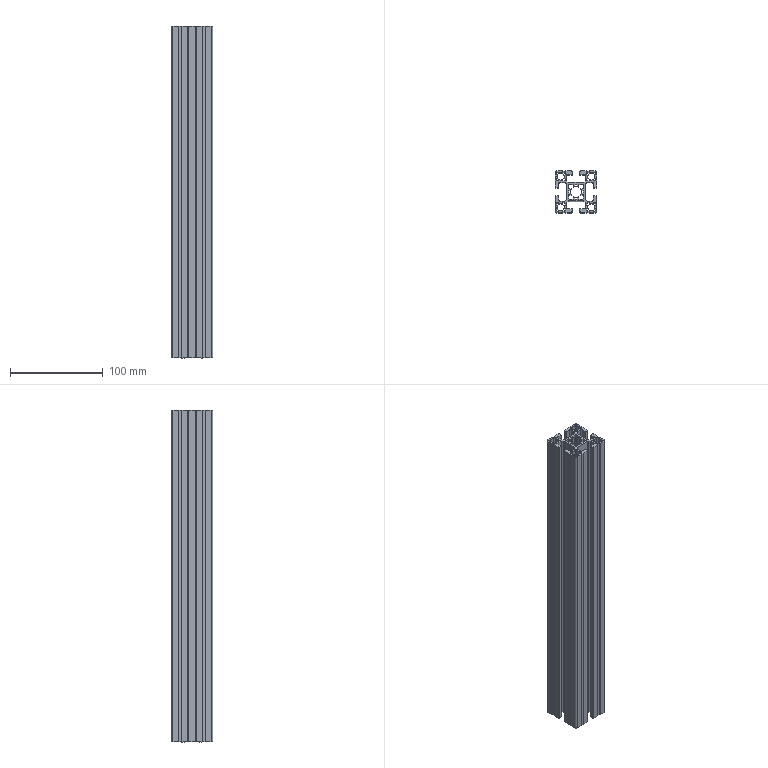Part | STEP file | 4545-400 aluminium profile (computer rack assembly 2) | 1 solid | 262 faces | box 45 x 45 x 358 mm | volume 248397 mm3 | plane 186 | cylinder 76 | commonest cylinder face diameters 2 x44 8 x20 12 x8 4 x4